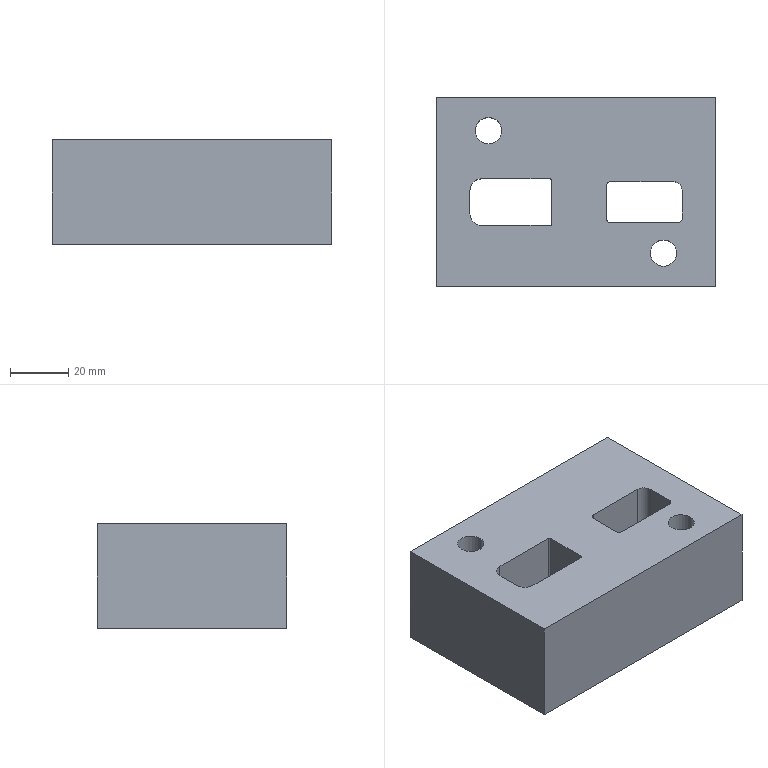Part | 1 solid | 40 faces | box 96 x 65 x 36 mm | volume 187629 mm3 | cylinder 20 | plane 16 | cone 4 | commonest cylinder face diameters 8 x6 9 x4 14 x4 3 x3 1 x2 6 x1